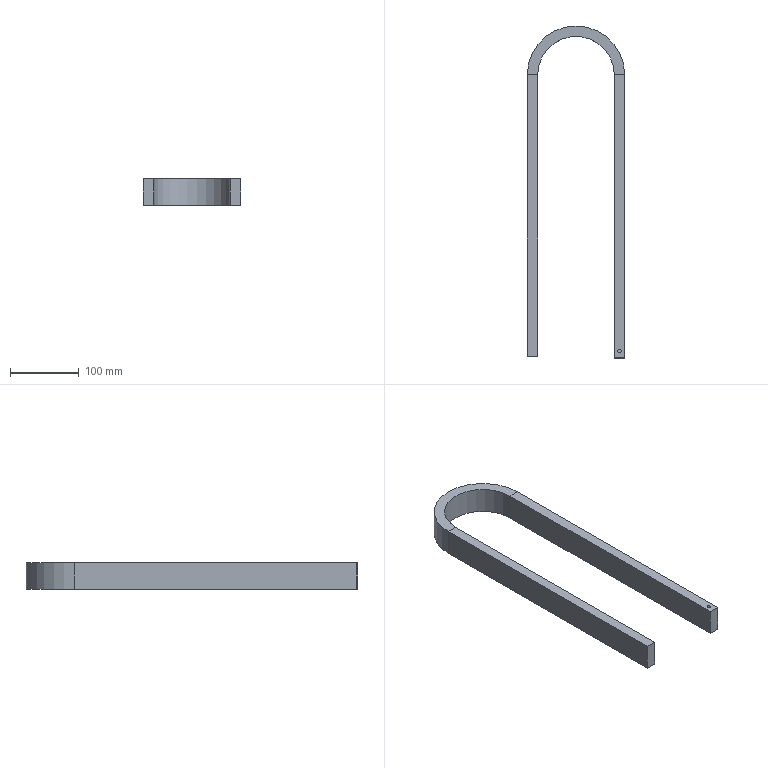Part | SolidWorks | features BaseBody 1 | 1 solid | 17 faces | box 141.75 x 483.375 x 38.9 mm | volume 599384 mm3 | plane 13 | cylinder 4 | commonest cylinder face diameters 5.2 x2 111.57 x1 141.75 x1
STEP:
#1=CARTESIAN_POINT('',(124.06,7.5,9.45));
#2=VERTEX_POINT('',#1);
#3=CARTESIAN_POINT('',(129.26,7.5,9.45));
#4=VERTEX_POINT('',#3);
#5=CARTESIAN_POINT('',(126.66,7.5,9.45));
#6=DIRECTION('',(0.,0.,1.));
#7=DIRECTION('',(1.,0.,0.));
#8=AXIS2_PLACEMENT_3D('',#5,#6,#7);
#9=CIRCLE('',#8,2.6);
#10=EDGE_CURVE('',#2,#4,#9,.T.);
#11=ORIENTED_EDGE('',*,*,#10,.F.);
#12=CARTESIAN_POINT('',(124.06,7.5,19.45));
#13=VERTEX_POINT('',#12);
#14=CARTESIAN_POINT('',(124.06,7.5,9.45));
#15=DIRECTION('',(0.,0.,1.));
#16=VECTOR('',#15,1000.);
#17=LINE('',#14,#16);
#18=EDGE_CURVE('',#2,#13,#17,.T.);
#19=ORIENTED_EDGE('',*,*,#18,.T.);
#20=CARTESIAN_POINT('',(129.26,7.5,19.45));
#21=VERTEX_POINT('',#20);
#22=CARTESIAN_POINT('',(126.66,7.5,19.45));
#23=DIRECTION('',(0.,0.,1.));
#24=DIRECTION('',(1.,0.,0.));
#25=AXIS2_PLACEMENT_3D('',#22,#23,#24);
#26=CIRCLE('',#25,2.6);
#27=EDGE_CURVE('',#13,#21,#26,.T.);
#28=ORIENTED_EDGE('',*,*,#27,.T.);
#29=CARTESIAN_POINT('',(129.26,7.5,9.45));
#30=DIRECTION('',(0.,0.,1.));
#31=VECTOR('',#30,1000.);
#32=LINE('',#29,#31);
#33=EDGE_CURVE('',#4,#21,#32,.T.);
#34=ORIENTED_EDGE('',*,*,#33,.F.);
#35=EDGE_LOOP('',(#11,#19,#28,#34));
#36=FACE_OUTER_BOUND('',#35,.T.);
#37=CARTESIAN_POINT('',(126.66,7.5,9.45));
#38=DIRECTION('',(0.,0.,1.));
#39=DIRECTION('',(1.,0.,0.));
#40=AXIS2_PLACEMENT_3D('',#37,#38,#39);
#41=CYLINDRICAL_SURFACE('',#40,2.6);
#42=ADVANCED_FACE('',(#36),#41,.F.);
#43=CARTESIAN_POINT('',(119.115,-2.5,-19.45));
#44=VERTEX_POINT('',#43);
#45=CARTESIAN_POINT('',(134.205,-2.5,-19.45));
#46=VERTEX_POINT('',#45);
#47=CARTESIAN_POINT('',(134.205,-2.5,-19.45));
#48=DIRECTION('',(1.,0.,0.));
#49=VECTOR('',#48,1000.);
#50=LINE('',#47,#49);
#51=EDGE_CURVE('',#44,#46,#50,.T.);
#52=ORIENTED_EDGE('',*,*,#51,.F.);
#53=CARTESIAN_POINT('',(119.115,410.,-19.45));
#54=VERTEX_POINT('',#53);
#55=CARTESIAN_POINT('',(119.115,410.,-19.45));
#56=DIRECTION('',(0.,-1.,0.));
#57=VECTOR('',#56,1000.);
#58=LINE('',#55,#57);
#59=EDGE_CURVE('',#54,#44,#58,.T.);
#60=ORIENTED_EDGE('',*,*,#59,.F.);
#61=CARTESIAN_POINT('',(134.205,410.,-19.45));
#62=VERTEX_POINT('',#61);
#63=CARTESIAN_POINT('',(134.205,410.,-19.45));
#64=DIRECTION('',(1.,0.,0.));
#65=VECTOR('',#64,1000.);
#66=LINE('',#63,#65);
#67=EDGE_CURVE('',#54,#62,#66,.T.);
#68=ORIENTED_EDGE('',*,*,#67,.T.);
#69=CARTESIAN_POINT('',(134.205,410.,-19.45));
#70=DIRECTION('',(0.,-1.,0.));
#71=VECTOR('',#70,1000.);
#72=LINE('',#69,#71);
#73=EDGE_CURVE('',#62,#46,#72,.T.);
#74=ORIENTED_EDGE('',*,*,#73,.T.);
#75=EDGE_LOOP('',(#52,#60,#68,#74));
#76=FACE_OUTER_BOUND('',#75,.T.);
#77=CARTESIAN_POINT('',(134.205,410.,-19.45));
#78=DIRECTION('',(0.,0.,-1.));
#79=DIRECTION('',(-1.,0.,0.));
#80=AXIS2_PLACEMENT_3D('',#77,#78,#79);
#81=PLANE('',#80);
#82=ADVANCED_FACE('',(#76),#81,.T.);
#83=ORIENTED_EDGE('',*,*,#59,.T.);
#84=CARTESIAN_POINT('',(119.115,-2.5,19.45));
#85=VERTEX_POINT('',#84);
#86=CARTESIAN_POINT('',(119.115,-2.5,-19.45));
#87=DIRECTION('',(0.,0.,-1.));
#88=VECTOR('',#87,1000.);
#89=LINE('',#86,#88);
#90=EDGE_CURVE('',#85,#44,#89,.T.);
#91=ORIENTED_EDGE('',*,*,#90,.F.);
#92=CARTESIAN_POINT('',(119.115,410.,19.45));
#93=VERTEX_POINT('',#92);
#94=CARTESIAN_POINT('',(119.115,410.,19.45));
#95=DIRECTION('',(0.,-1.,0.));
#96=VECTOR('',#95,1000.);
#97=LINE('',#94,#96);
#98=EDGE_CURVE('',#93,#85,#97,.T.);
#99=ORIENTED_EDGE('',*,*,#98,.F.);
#100=CARTESIAN_POINT('',(119.115,410.,-19.45));
#101=DIRECTION('',(0.,0.,-1.));
#102=VECTOR('',#101,1000.);
#103=LINE('',#100,#102);
#104=EDGE_CURVE('',#93,#54,#103,.T.);
#105=ORIENTED_EDGE('',*,*,#104,.T.);
#106=EDGE_LOOP('',(#83,#91,#99,#105));
#107=FACE_OUTER_BOUND('',#106,.T.);
#108=CARTESIAN_POINT('',(119.115,410.,-19.45));
#109=DIRECTION('',(-1.,0.,0.));
#110=DIRECTION('',(0.,-1.,0.));
#111=AXIS2_PLACEMENT_3D('',#108,#109,#110);
#112=PLANE('',#111);
#113=ADVANCED_FACE('',(#107),#112,.T.);
#114=CARTESIAN_POINT('',(126.66,7.5,19.45));
#115=DIRECTION('',(0.,0.,1.));
#116=DIRECTION('',(1.,0.,0.));
#117=AXIS2_PLACEMENT_3D('',#114,#115,#116);
#118=CIRCLE('',#117,2.6);
#119=EDGE_CURVE('',#21,#13,#118,.T.);
#120=ORIENTED_EDGE('',*,*,#119,.F.);
#121=ORIENTED_EDGE('',*,*,#27,.F.);
#122=EDGE_LOOP('',(#120,#121));
#123=FACE_BOUND('',#122,.T.);
#124=ORIENTED_EDGE('',*,*,#98,.T.);
#125=CARTESIAN_POINT('',(134.205,-2.5,19.45));
#126=VERTEX_POINT('',#125);
#127=CARTESIAN_POINT('',(134.205,-2.5,19.45));
#128=DIRECTION('',(-1.,0.,0.));
#129=VECTOR('',#128,1000.);
#130=LINE('',#127,#129);
#131=EDGE_CURVE('',#126,#85,#130,.T.);
#132=ORIENTED_EDGE('',*,*,#131,.F.);
#133=CARTESIAN_POINT('',(134.205,410.,19.45));
#134=VERTEX_POINT('',#133);
#135=CARTESIAN_POINT('',(134.205,410.,19.45));
#136=DIRECTION('',(0.,-1.,0.));
#137=VECTOR('',#136,1000.);
#138=LINE('',#135,#137);
#139=EDGE_CURVE('',#134,#126,#138,.T.);
#140=ORIENTED_EDGE('',*,*,#139,.F.);
#141=CARTESIAN_POINT('',(134.205,410.,19.45));
#142=DIRECTION('',(-1.,0.,0.));
#143=VECTOR('',#142,1000.);
#144=LINE('',#141,#143);
#145=EDGE_CURVE('',#134,#93,#144,.T.);
#146=ORIENTED_EDGE('',*,*,#145,.T.);
#147=EDGE_LOOP('',(#124,#132,#140,#146));
#148=FACE_OUTER_BOUND('',#147,.T.);
#149=CARTESIAN_POINT('',(134.205,410.,19.45));
#150=DIRECTION('',(0.,0.,1.));
#151=DIRECTION('',(1.,0.,0.));
#152=AXIS2_PLACEMENT_3D('',#149,#150,#151);
#153=PLANE('',#152);
#154=ADVANCED_FACE('',(#123,#148),#153,.T.);
#155=ORIENTED_EDGE('',*,*,#139,.T.);
#156=CARTESIAN_POINT('',(134.205,-2.5,-19.45));
#157=DIRECTION('',(0.,0.,1.));
#158=VECTOR('',#157,1000.);
#159=LINE('',#156,#158);
#160=EDGE_CURVE('',#46,#126,#159,.T.);
#161=ORIENTED_EDGE('',*,*,#160,.F.);
#162=ORIENTED_EDGE('',*,*,#73,.F.);
#163=CARTESIAN_POINT('',(134.205,410.,-19.45));
#164=DIRECTION('',(0.,0.,1.));
#165=VECTOR('',#164,1000.);
#166=LINE('',#163,#165);
#167=EDGE_CURVE('',#62,#134,#166,.T.);
#168=ORIENTED_EDGE('',*,*,#167,.T.);
#169=EDGE_LOOP('',(#155,#161,#162,#168));
#170=FACE_OUTER_BOUND('',#169,.T.);
#171=CARTESIAN_POINT('',(134.205,410.,-19.45));
#172=DIRECTION('',(1.,0.,0.));
#173=DIRECTION('',(0.,1.,0.));
#174=AXIS2_PLACEMENT_3D('',#171,#172,#173);
#175=PLANE('',#174);
#176=ADVANCED_FACE('',(#170),#175,.T.);
#177=ORIENTED_EDGE('',*,*,#67,.F.);
#178=CARTESIAN_POINT('',(7.545,410.,-19.45));
#179=VERTEX_POINT('',#178);
#180=CARTESIAN_POINT('',(63.33,410.,-19.45));
#181=DIRECTION('',(0.,0.,-1.));
#182=DIRECTION('',(-1.,0.,0.));
#183=AXIS2_PLACEMENT_3D('',#180,#181,#182);
#184=CIRCLE('',#183,55.785);
#185=EDGE_CURVE('',#179,#54,#184,.T.);
#186=ORIENTED_EDGE('',*,*,#185,.F.);
#187=CARTESIAN_POINT('',(-7.545,410.,-19.45));
#188=VERTEX_POINT('',#187);
#189=CARTESIAN_POINT('',(-7.545,410.,-19.45));
#190=DIRECTION('',(-1.,0.,0.));
#191=VECTOR('',#190,1000.);
#192=LINE('',#189,#191);
#193=EDGE_CURVE('',#179,#188,#192,.T.);
#194=ORIENTED_EDGE('',*,*,#193,.T.);
#195=CARTESIAN_POINT('',(63.33,410.,-19.45));
#196=DIRECTION('',(0.,0.,-1.));
#197=DIRECTION('',(-1.,0.,0.));
#198=AXIS2_PLACEMENT_3D('',#195,#196,#197);
#199=CIRCLE('',#198,70.875);
#200=EDGE_CURVE('',#188,#62,#199,.T.);
#201=ORIENTED_EDGE('',*,*,#200,.T.);
#202=EDGE_LOOP('',(#177,#186,#194,#201));
#203=FACE_OUTER_BOUND('',#202,.T.);
#204=CARTESIAN_POINT('',(-7.545,410.,-19.45));
#205=DIRECTION('',(0.,0.,-1.));
#206=DIRECTION('',(-1.,0.,0.));
#207=AXIS2_PLACEMENT_3D('',#204,#205,#206);
#208=PLANE('',#207);
#209=ADVANCED_FACE('',(#203),#208,.T.);
#210=ORIENTED_EDGE('',*,*,#185,.T.);
#211=ORIENTED_EDGE('',*,*,#104,.F.);
#212=CARTESIAN_POINT('',(7.545,410.,19.45));
#213=VERTEX_POINT('',#212);
#214=CARTESIAN_POINT('',(63.33,410.,19.45));
#215=DIRECTION('',(0.,0.,-1.));
#216=DIRECTION('',(-1.,0.,0.));
#217=AXIS2_PLACEMENT_3D('',#214,#215,#216);
#218=CIRCLE('',#217,55.785);
#219=EDGE_CURVE('',#213,#93,#218,.T.);
#220=ORIENTED_EDGE('',*,*,#219,.F.);
#221=CARTESIAN_POINT('',(7.545,410.,-19.45));
#222=DIRECTION('',(0.,0.,-1.));
#223=VECTOR('',#222,1000.);
#224=LINE('',#221,#223);
#225=EDGE_CURVE('',#213,#179,#224,.T.);
#226=ORIENTED_EDGE('',*,*,#225,.T.);
#227=EDGE_LOOP('',(#210,#211,#220,#226));
#228=FACE_OUTER_BOUND('',#227,.T.);
#229=CARTESIAN_POINT('',(63.33,410.,0.));
#230=DIRECTION('',(0.,0.,-1.));
#231=DIRECTION('',(-1.,0.,0.));
#232=AXIS2_PLACEMENT_3D('',#229,#230,#231);
#233=CYLINDRICAL_SURFACE('',#232,55.785);
#234=ADVANCED_FACE('',(#228),#233,.F.);
#235=ORIENTED_EDGE('',*,*,#219,.T.);
#236=ORIENTED_EDGE('',*,*,#145,.F.);
#237=CARTESIAN_POINT('',(-7.545,410.,19.45));
#238=VERTEX_POINT('',#237);
#239=CARTESIAN_POINT('',(63.33,410.,19.45));
#240=DIRECTION('',(0.,0.,-1.));
#241=DIRECTION('',(-1.,0.,0.));
#242=AXIS2_PLACEMENT_3D('',#239,#240,#241);
#243=CIRCLE('',#242,70.875);
#244=EDGE_CURVE('',#238,#134,#243,.T.);
#245=ORIENTED_EDGE('',*,*,#244,.F.);
#246=CARTESIAN_POINT('',(-7.545,410.,19.45));
#247=DIRECTION('',(1.,0.,0.));
#248=VECTOR('',#247,1000.);
#249=LINE('',#246,#248);
#250=EDGE_CURVE('',#238,#213,#249,.T.);
#251=ORIENTED_EDGE('',*,*,#250,.T.);
#252=EDGE_LOOP('',(#235,#236,#245,#251));
#253=FACE_OUTER_BOUND('',#252,.T.);
#254=CARTESIAN_POINT('',(-7.545,410.,19.45));
#255=DIRECTION('',(0.,0.,1.));
#256=DIRECTION('',(1.,0.,0.));
#257=AXIS2_PLACEMENT_3D('',#254,#255,#256);
#258=PLANE('',#257);
#259=ADVANCED_FACE('',(#253),#258,.T.);
#260=ORIENTED_EDGE('',*,*,#244,.T.);
#261=ORIENTED_EDGE('',*,*,#167,.F.);
#262=ORIENTED_EDGE('',*,*,#200,.F.);
#263=CARTESIAN_POINT('',(-7.545,410.,-19.45));
#264=DIRECTION('',(0.,0.,1.));
#265=VECTOR('',#264,1000.);
#266=LINE('',#263,#265);
#267=EDGE_CURVE('',#188,#238,#266,.T.);
#268=ORIENTED_EDGE('',*,*,#267,.T.);
#269=EDGE_LOOP('',(#260,#261,#262,#268));
#270=FACE_OUTER_BOUND('',#269,.T.);
#271=CARTESIAN_POINT('',(63.33,410.,0.));
#272=DIRECTION('',(0.,0.,-1.));
#273=DIRECTION('',(-1.,0.,0.));
#274=AXIS2_PLACEMENT_3D('',#271,#272,#273);
#275=CYLINDRICAL_SURFACE('',#274,70.875);
#276=ADVANCED_FACE('',(#270),#275,.T.);
#277=ORIENTED_EDGE('',*,*,#193,.F.);
#278=CARTESIAN_POINT('',(7.545,0.,-19.45));
#279=VERTEX_POINT('',#278);
#280=CARTESIAN_POINT('',(7.545,0.,-19.45));
#281=DIRECTION('',(0.,1.,0.));
#282=VECTOR('',#281,1000.);
#283=LINE('',#280,#282);
#284=EDGE_CURVE('',#279,#179,#283,.T.);
#285=ORIENTED_EDGE('',*,*,#284,.F.);
#286=CARTESIAN_POINT('',(-7.545,0.,-19.45));
#287=VERTEX_POINT('',#286);
#288=CARTESIAN_POINT('',(-7.545,0.,-19.45));
#289=DIRECTION('',(-1.,0.,0.));
#290=VECTOR('',#289,1000.);
#291=LINE('',#288,#290);
#292=EDGE_CURVE('',#279,#287,#291,.T.);
#293=ORIENTED_EDGE('',*,*,#292,.T.);
#294=CARTESIAN_POINT('',(-7.545,0.,-19.45));
#295=DIRECTION('',(0.,1.,0.));
#296=VECTOR('',#295,1000.);
#297=LINE('',#294,#296);
#298=EDGE_CURVE('',#287,#188,#297,.T.);
#299=ORIENTED_EDGE('',*,*,#298,.T.);
#300=EDGE_LOOP('',(#277,#285,#293,#299));
#301=FACE_OUTER_BOUND('',#300,.T.);
#302=CARTESIAN_POINT('',(-7.545,0.,-19.45));
#303=DIRECTION('',(0.,0.,-1.));
#304=DIRECTION('',(-1.,0.,0.));
#305=AXIS2_PLACEMENT_3D('',#302,#303,#304);
#306=PLANE('',#305);
#307=ADVANCED_FACE('',(#301),#306,.T.);
#308=ORIENTED_EDGE('',*,*,#284,.T.);
#309=ORIENTED_EDGE('',*,*,#225,.F.);
#310=CARTESIAN_POINT('',(7.545,0.,19.45));
#311=VERTEX_POINT('',#310);
#312=CARTESIAN_POINT('',(7.545,0.,19.45));
#313=DIRECTION('',(0.,1.,0.));
#314=VECTOR('',#313,1000.);
#315=LINE('',#312,#314);
#316=EDGE_CURVE('',#311,#213,#315,.T.);
#317=ORIENTED_EDGE('',*,*,#316,.F.);
#318=CARTESIAN_POINT('',(7.545,0.,-19.45));
#319=DIRECTION('',(0.,0.,-1.));
#320=VECTOR('',#319,1000.);
#321=LINE('',#318,#320);
#322=EDGE_CURVE('',#311,#279,#321,.T.);
#323=ORIENTED_EDGE('',*,*,#322,.T.);
#324=EDGE_LOOP('',(#308,#309,#317,#323));
#325=FACE_OUTER_BOUND('',#324,.T.);
#326=CARTESIAN_POINT('',(7.545,0.,-19.45));
#327=DIRECTION('',(1.,0.,0.));
#328=DIRECTION('',(0.,0.,-1.));
#329=AXIS2_PLACEMENT_3D('',#326,#327,#328);
#330=PLANE('',#329);
#331=ADVANCED_FACE('',(#325),#330,.T.);
#332=ORIENTED_EDGE('',*,*,#316,.T.);
#333=ORIENTED_EDGE('',*,*,#250,.F.);
#334=CARTESIAN_POINT('',(-7.545,0.,19.45));
#335=VERTEX_POINT('',#334);
#336=CARTESIAN_POINT('',(-7.545,0.,19.45));
#337=DIRECTION('',(0.,1.,0.));
#338=VECTOR('',#337,1000.);
#339=LINE('',#336,#338);
#340=EDGE_CURVE('',#335,#238,#339,.T.);
#341=ORIENTED_EDGE('',*,*,#340,.F.);
#342=CARTESIAN_POINT('',(-7.545,0.,19.45));
#343=DIRECTION('',(1.,0.,0.));
#344=VECTOR('',#343,1000.);
#345=LINE('',#342,#344);
#346=EDGE_CURVE('',#335,#311,#345,.T.);
#347=ORIENTED_EDGE('',*,*,#346,.T.);
#348=EDGE_LOOP('',(#332,#333,#341,#347));
#349=FACE_OUTER_BOUND('',#348,.T.);
#350=CARTESIAN_POINT('',(-7.545,0.,19.45));
#351=DIRECTION('',(0.,0.,1.));
#352=DIRECTION('',(1.,0.,0.));
#353=AXIS2_PLACEMENT_3D('',#350,#351,#352);
#354=PLANE('',#353);
#355=ADVANCED_FACE('',(#349),#354,.T.);
#356=ORIENTED_EDGE('',*,*,#340,.T.);
#357=ORIENTED_EDGE('',*,*,#267,.F.);
#358=ORIENTED_EDGE('',*,*,#298,.F.);
#359=CARTESIAN_POINT('',(-7.545,0.,-19.45));
#360=DIRECTION('',(0.,0.,1.));
#361=VECTOR('',#360,1000.);
#362=LINE('',#359,#361);
#363=EDGE_CURVE('',#287,#335,#362,.T.);
#364=ORIENTED_EDGE('',*,*,#363,.T.);
#365=EDGE_LOOP('',(#356,#357,#358,#364));
#366=FACE_OUTER_BOUND('',#365,.T.);
#367=CARTESIAN_POINT('',(-7.545,0.,-19.45));
#368=DIRECTION('',(-1.,0.,0.));
#369=DIRECTION('',(0.,0.,1.));
#370=AXIS2_PLACEMENT_3D('',#367,#368,#369);
#371=PLANE('',#370);
#372=ADVANCED_FACE('',(#366),#371,.T.);
#373=ORIENTED_EDGE('',*,*,#90,.T.);
#374=ORIENTED_EDGE('',*,*,#51,.T.);
#375=ORIENTED_EDGE('',*,*,#160,.T.);
#376=ORIENTED_EDGE('',*,*,#131,.T.);
#377=EDGE_LOOP('',(#373,#374,#375,#376));
#378=FACE_OUTER_BOUND('',#377,.T.);
#379=CARTESIAN_POINT('',(126.66,-2.5,0.));
#380=DIRECTION('',(0.,-1.,0.));
#381=DIRECTION('',(0.,0.,1.));
#382=AXIS2_PLACEMENT_3D('',#379,#380,#381);
#383=PLANE('',#382);
#384=ADVANCED_FACE('',(#378),#383,.T.);
#385=ORIENTED_EDGE('',*,*,#322,.F.);
#386=ORIENTED_EDGE('',*,*,#346,.F.);
#387=ORIENTED_EDGE('',*,*,#363,.F.);
#388=ORIENTED_EDGE('',*,*,#292,.F.);
#389=EDGE_LOOP('',(#385,#386,#387,#388));
#390=FACE_OUTER_BOUND('',#389,.T.);
#391=CARTESIAN_POINT('',(0.,0.,0.));
#392=DIRECTION('',(0.,1.,0.));
#393=DIRECTION('',(0.,0.,1.));
#394=AXIS2_PLACEMENT_3D('',#391,#392,#393);
#395=PLANE('',#394);
#396=ADVANCED_FACE('',(#390),#395,.F.);
#397=ORIENTED_EDGE('',*,*,#18,.F.);
#398=CARTESIAN_POINT('',(126.66,7.5,9.45));
#399=DIRECTION('',(0.,0.,1.));
#400=DIRECTION('',(1.,0.,0.));
#401=AXIS2_PLACEMENT_3D('',#398,#399,#400);
#402=CIRCLE('',#401,2.6);
#403=EDGE_CURVE('',#4,#2,#402,.T.);
#404=ORIENTED_EDGE('',*,*,#403,.F.);
#405=ORIENTED_EDGE('',*,*,#33,.T.);
#406=ORIENTED_EDGE('',*,*,#119,.T.);
#407=EDGE_LOOP('',(#397,#404,#405,#406));
#408=FACE_OUTER_BOUND('',#407,.T.);
#409=CARTESIAN_POINT('',(126.66,7.5,9.45));
#410=DIRECTION('',(0.,0.,1.));
#411=DIRECTION('',(1.,0.,0.));
#412=AXIS2_PLACEMENT_3D('',#409,#410,#411);
#413=CYLINDRICAL_SURFACE('',#412,2.6);
#414=ADVANCED_FACE('',(#408),#413,.F.);
#415=ORIENTED_EDGE('',*,*,#403,.T.);
#416=ORIENTED_EDGE('',*,*,#10,.T.);
#417=EDGE_LOOP('',(#415,#416));
#418=FACE_OUTER_BOUND('',#417,.T.);
#419=CARTESIAN_POINT('',(126.66,7.5,9.45));
#420=DIRECTION('',(0.,0.,1.));
#421=DIRECTION('',(1.,0.,0.));
#422=AXIS2_PLACEMENT_3D('',#419,#420,#421);
#423=PLANE('',#422);
#424=ADVANCED_FACE('',(#418),#423,.T.);
#425=CLOSED_SHELL('',(#42,#82,#113,#154,#176,#209,#234,#259,#276,#307,#331,#355,#372,#384,#396,#414,#424));
#426=MANIFOLD_SOLID_BREP('',#425);
#427=CARTESIAN_POINT('',(0.,0.,0.));
#428=DIRECTION('',(0.,0.,1.));
#429=DIRECTION('',(1.,0.,0.));
#430=AXIS2_PLACEMENT_3D('',#427,#428,#429);
#431=(LENGTH_UNIT()NAMED_UNIT(*)SI_UNIT(.MILLI.,.METRE.));
#432=UNCERTAINTY_MEASURE_WITH_UNIT(LENGTH_MEASURE(0.00001),#431,'','');
#433=(NAMED_UNIT(*)PLANE_ANGLE_UNIT()SI_UNIT($,.RADIAN.));
#434=(NAMED_UNIT(*)SI_UNIT($,.STERADIAN.)SOLID_ANGLE_UNIT());
#435=(GEOMETRIC_REPRESENTATION_CONTEXT(3)GLOBAL_UNCERTAINTY_ASSIGNED_CONTEXT((#432))GLOBAL_UNIT_ASSIGNED_CONTEXT((#431,#433,#434))REPRESENTATION_CONTEXT('',''));
#436=ADVANCED_BREP_SHAPE_REPRESENTATION('',(#426,#430),#435);